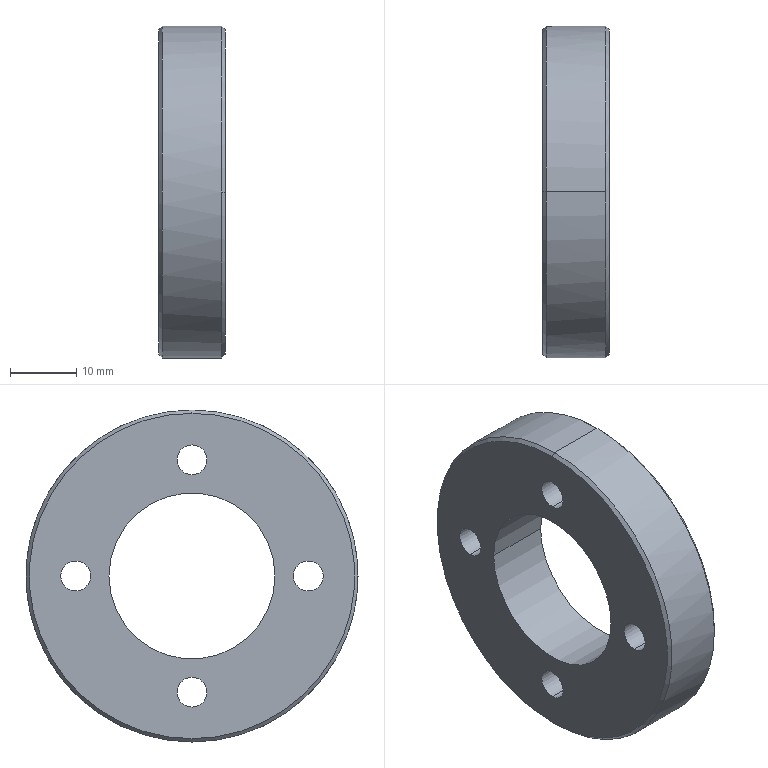Part | STEP file | 06-22 Stator support plate | 1 solid | 30 faces | box 10 x 50 x 50 mm | volume 13234 mm3 | cylinder 20 | plane 6 | cone 4 | commonest cylinder face diameters 4.5 x8 8.5 x8 25 x2 50 x2